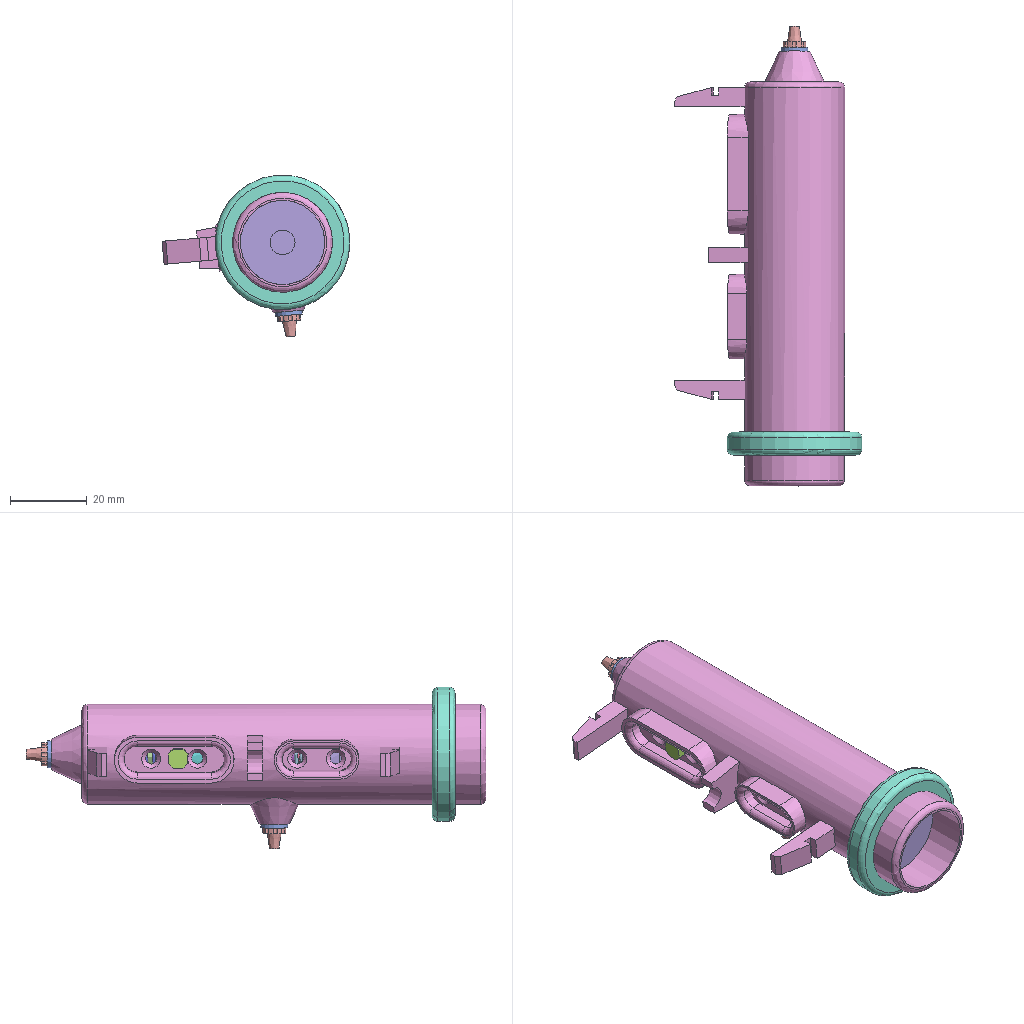Assembly | NX | 15 different items | 19 placed | box 49 x 120 x 42 mm
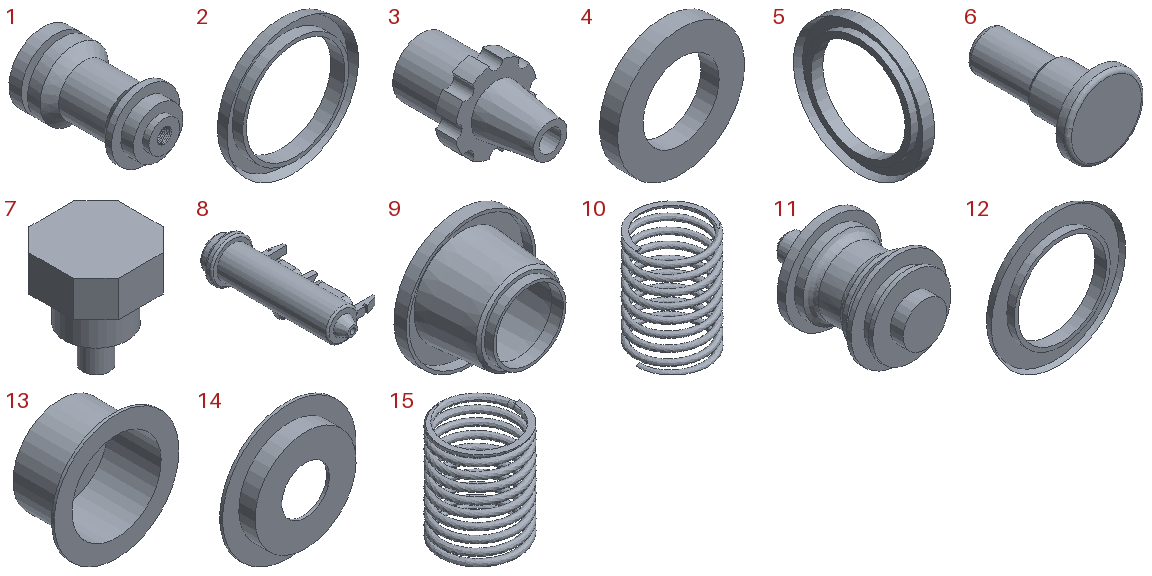Parts list (item | quantity | size | volume | features):
1 | x1 | 22 x 39 x 22 mm | 9431 mm3 | features DATUM_CSYS 9, EXTRUDE 8, SKETCH 8, CHAMFER 2, THREADS 1
2 | x1 | 21.341 x 2.3 x 21.341 mm | 152.879 mm3 | features DATUM_CSYS 3, SKETCH 2, SWP104 1
3 | x2 | 5.92 x 9.5 x 5.92 mm | 103.972 mm3 | features EXTRUDE 12, EXTRACT_STRING 8, Instance Feature 7, DATUM_CSYS 5, SKETCH 4, DRAFT 1, Pattern Feature 1, SYMBOLIC_THREAD 1
4 | x2 | 7 x 1 x 7 mm | 24.63 mm3 | features DATUM_CSYS 2, EXTRUDE 1, SKETCH 1
5 | x3 | 2 x 22 x 22 mm | 223.441 mm3 | features DATUM_CSYS 3, SKETCH 2, SWP104 1
6 | x1 | 10 x 15.5 x 10 mm | 439.857 mm3 | features DATUM_CSYS 4, EXTRUDE 3, SKETCH 3, BLEND 2, CHAMFER 1
7 | x1 | 5 x 4.979 x 6 mm | 66.325 mm3 | features DATUM_CSYS 4, EXTRUDE 3, SKETCH 3, SYMBOLIC_THREAD 1
8 | x1 | 48.659 x 113 x 35.5 mm | 22611 mm3 | features EXTRUDE 29, DATUM_CSYS 24, SKETCH 23, BLEND 5, CHAMFER 5, SYMBOLIC_THREAD 3, DRAFT 2
9 | x1 | 13.6 x 7.451 x 13.6 mm | 99.127 mm3 | features DATUM_CSYS 3, SKETCH 2, SWP104 1
10 | x1 | - | 252.111 mm3 | features SPLINE_LAW 3, BRIDGE_CURVE 2, DATUM_CSYS 2, DATUM_PLANE 2, TRIM BODY 2, ABSOLUTE_DATUM_AXIS 1, ABSOLUTE_DATUM_PLANE 1, DATUM_ON_PATH 1, FLEXIBLE_PART 1, FSET 1, SKETCH 1, SKIN 1
11 | x1 | 22 x 32 x 22 mm | 5202 mm3 | features EXTRUDE 11, DATUM_CSYS 8, SKETCH 7, BLEND 3, CHAMFER 1
12 | x1 | 21.26 x 1.8 x 21.26 mm | 144.963 mm3 | features DATUM_CSYS 2, SKETCH 1, SWP104 1
13 | x1 | 14 x 6.3 x 14 mm | 95.944 mm3 | features DATUM_CSYS 2, SKETCH 1, SWP104 1
14 | x1 | 14 x 2 x 14 mm | 56.794 mm3 | features DATUM_CSYS 3, SKETCH 2, SWP104 1
15 | x1 | - | 283.448 mm3 | features SPLINE_LAW 3, BRIDGE_CURVE 2, DATUM_CSYS 2, DATUM_PLANE 2, TRIM BODY 2, ABSOLUTE_DATUM_AXIS 1, ABSOLUTE_DATUM_PLANE 1, DATUM_ON_PATH 1, FLEXIBLE_PART 1, FSET 1, SKETCH 1, SKIN 1
Mates (type | each side: item.copy, entity, surface, feature):
Touch | 4.1 face plane Extrude(2) | 3.1 face plane Extrude(4) | 2 times
Touch | 4.1 face plane Extrude(2) | 8.1 face plane Extrude(22)
Touch | 4.1 face plane Extrude(2) | 8.1 face plane Extrude(33)
Touch | 12.1 face plane Revolve(2) | 11.1 face plane Extrude(2)
Touch | 7.1 face plane Extrude(2) | 8.1 face plane Extrude(44)
Touch | 9.1 face plane Revolve(3) | 11.1 face plane Extrude(2)
Touch | 2.1 face plane Revolve(3) | 1.1 face plane Extrude(4)
Bond | 5.1 component | 1.1 component
Touch | 1.1 face plane Extrude(2) | 14.1 face plane Revolve(3)